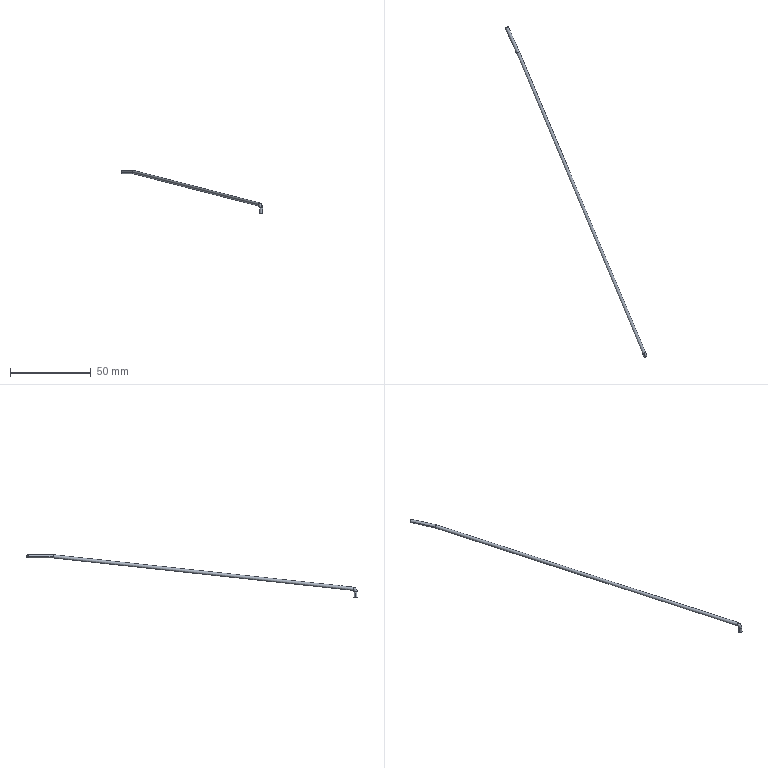Part | STEP file | rear_spoke5 | 1 solid | 10 faces | box 87.859 x 205.125 x 26.5 mm | volume 711.916 mm3 | cylinder 6 | torus 2 | plane 2 | commonest cylinder face diameters 2 x6
STEP:
#1=CARTESIAN_POINT('',(0.,0.,0.));
#2=DIRECTION('',(0.,0.,1.));
#3=DIRECTION('',(1.,0.,0.));
#4=AXIS2_PLACEMENT_3D('',#1,#2,#3);
#5=CARTESIAN_POINT('',(-17.112,24.113,0.3593));
#6=VERTEX_POINT('',#5);
#7=CARTESIAN_POINT('',(-15.725,23.191,0.3593));
#8=VERTEX_POINT('',#7);
#9=CARTESIAN_POINT('',(-16.112,24.113,0.3593));
#10=DIRECTION('',(0.,0.,1.));
#11=DIRECTION('',(1.,0.,0.));
#12=AXIS2_PLACEMENT_3D('',#9,#10,#11);
#13=CIRCLE('',#12,1.);
#14=CARTESIAN_POINT('',(-16.886,25.957,0.3593));
#15=DIRECTION('',(-0.9221,-0.387,0.));
#16=DIRECTION('',(0.387,-0.9221,0.));
#17=AXIS2_PLACEMENT_3D('',#14,#15,#16);
#18=TOROIDAL_SURFACE('',#17,2.,1.);
#19=CARTESIAN_POINT('',(0.,5.11));
#20=DIRECTION('',(0.,-1.));
#21=VECTOR('',#20,1.);
#22=LINE('',#19,#21);
#23=(GEOMETRIC_REPRESENTATION_CONTEXT(2)PARAMETRIC_REPRESENTATION_CONTEXT()REPRESENTATION_CONTEXT('',''));
#24=DEFINITIONAL_REPRESENTATION('',(#22),#23);
#25=PCURVE('',#18,#24);
#26=CARTESIAN_POINT('',(-16.112,24.113,-3.));
#27=DIRECTION('',(0.,0.,1.));
#28=DIRECTION('',(1.,0.,0.));
#29=AXIS2_PLACEMENT_3D('',#26,#27,#28);
#30=CYLINDRICAL_SURFACE('',#29,1.);
#31=CARTESIAN_POINT('',(0.,3.359));
#32=DIRECTION('',(1.,0.));
#33=VECTOR('',#32,1.);
#34=LINE('',#31,#33);
#35=(GEOMETRIC_REPRESENTATION_CONTEXT(2)PARAMETRIC_REPRESENTATION_CONTEXT()REPRESENTATION_CONTEXT('',''));
#36=DEFINITIONAL_REPRESENTATION('',(#34),#35);
#37=PCURVE('',#30,#36);
#38=SURFACE_CURVE('',#13,(#25,#37),.PCURVE_S1.);
#39=EDGE_CURVE('',#6,#8,#38,.T.);
#40=ORIENTED_EDGE('',*,*,#39,.T.);
#41=CARTESIAN_POINT('',(-16.771,25.683,3.345));
#42=VERTEX_POINT('',#41);
#43=CARTESIAN_POINT('',(-16.886,25.957,0.3593));
#44=DIRECTION('',(-0.9221,-0.387,0.));
#45=DIRECTION('',(0.387,-0.9221,0.));
#46=AXIS2_PLACEMENT_3D('',#43,#44,#45);
#47=CIRCLE('',#46,3.);
#48=CARTESIAN_POINT('',(0.,0.));
#49=DIRECTION('',(1.,0.));
#50=VECTOR('',#49,1.);
#51=LINE('',#48,#50);
#52=(GEOMETRIC_REPRESENTATION_CONTEXT(2)PARAMETRIC_REPRESENTATION_CONTEXT()REPRESENTATION_CONTEXT('',''));
#53=DEFINITIONAL_REPRESENTATION('',(#51),#52);
#54=PCURVE('',#18,#53);
#55=CARTESIAN_POINT('',(-16.886,25.957,0.3593));
#56=DIRECTION('',(-0.9221,-0.387,0.));
#57=DIRECTION('',(0.387,-0.9221,0.));
#58=AXIS2_PLACEMENT_3D('',#55,#56,#57);
#59=TOROIDAL_SURFACE('',#58,2.,1.);
#60=CARTESIAN_POINT('',(0.,6.283));
#61=CARTESIAN_POINT('',(0.0223,6.283));
#62=CARTESIAN_POINT('',(0.06689,6.283));
#63=CARTESIAN_POINT('',(0.1338,6.283));
#64=CARTESIAN_POINT('',(0.2007,6.283));
#65=CARTESIAN_POINT('',(0.2675,6.283));
#66=CARTESIAN_POINT('',(0.3344,6.283));
#67=CARTESIAN_POINT('',(0.4013,6.283));
#68=CARTESIAN_POINT('',(0.4682,6.283));
#69=CARTESIAN_POINT('',(0.5351,6.283));
#70=CARTESIAN_POINT('',(0.602,6.283));
#71=CARTESIAN_POINT('',(0.6689,6.283));
#72=CARTESIAN_POINT('',(0.7358,6.283));
#73=CARTESIAN_POINT('',(0.8026,6.283));
#74=CARTESIAN_POINT('',(0.8695,6.283));
#75=CARTESIAN_POINT('',(0.9364,6.283));
#76=CARTESIAN_POINT('',(1.003,6.283));
#77=CARTESIAN_POINT('',(1.07,6.283));
#78=CARTESIAN_POINT('',(1.137,6.283));
#79=CARTESIAN_POINT('',(1.204,6.283));
#80=CARTESIAN_POINT('',(1.271,6.283));
#81=CARTESIAN_POINT('',(1.338,6.283));
#82=CARTESIAN_POINT('',(1.405,6.283));
#83=CARTESIAN_POINT('',(1.449,6.283));
#84=CARTESIAN_POINT('',(1.472,6.283));
#85=B_SPLINE_CURVE_WITH_KNOTS('',3,(#60,#61,#62,#63,#64,#65,#66,#67,#68,#69,#70,#71,#72,#73,#74,#75,#76,#77,#78,#79,#80,#81,#82,#83,#84),.UNSPECIFIED.,.F.,.F.,(4,1,1,1,1,1,1,1,1,1,1,1,1,1,1,1,1,1,1,1,1,1,4),(0.,0.06689,0.1338,0.2007,0.2675,0.3344,0.4013,0.4682,0.5351,0.602,0.6689,0.7358,0.8026,0.8695,0.9364,1.003,1.07,1.137,1.204,1.271,1.338,1.405,1.472),.QUASI_UNIFORM_KNOTS.);
#86=(GEOMETRIC_REPRESENTATION_CONTEXT(2)PARAMETRIC_REPRESENTATION_CONTEXT()REPRESENTATION_CONTEXT('',''));
#87=DEFINITIONAL_REPRESENTATION('',(#85),#86);
#88=PCURVE('',#59,#87);
#89=SURFACE_CURVE('',#47,(#54,#88),.PCURVE_S1.);
#90=EDGE_CURVE('',#8,#42,#89,.T.);
#91=ORIENTED_EDGE('',*,*,#90,.T.);
#92=CARTESIAN_POINT('',(-17.731,25.387,2.349));
#93=VERTEX_POINT('',#92);
#94=CARTESIAN_POINT('',(-16.809,25.774,2.349));
#95=DIRECTION('',(-0.3851,0.9175,0.09911));
#96=DIRECTION('',(0.8651,0.3215,0.3851));
#97=AXIS2_PLACEMENT_3D('',#94,#95,#96);
#98=CIRCLE('',#97,1.);
#99=CARTESIAN_POINT('',(1.472,5.11));
#100=DIRECTION('',(0.,-1.));
#101=VECTOR('',#100,1.);
#102=LINE('',#99,#101);
#103=(GEOMETRIC_REPRESENTATION_CONTEXT(2)PARAMETRIC_REPRESENTATION_CONTEXT()REPRESENTATION_CONTEXT('',''));
#104=DEFINITIONAL_REPRESENTATION('',(#102),#103);
#105=PCURVE('',#18,#104);
#106=CARTESIAN_POINT('',(-16.809,25.774,2.349));
#107=DIRECTION('',(-0.3851,0.9175,0.09911));
#108=DIRECTION('',(-0.9221,-0.387,0.));
#109=AXIS2_PLACEMENT_3D('',#106,#107,#108);
#110=CYLINDRICAL_SURFACE('',#109,1.);
#111=CARTESIAN_POINT('',(-3.539,0.));
#112=DIRECTION('',(1.,0.));
#113=VECTOR('',#112,1.);
#114=LINE('',#111,#113);
#115=(GEOMETRIC_REPRESENTATION_CONTEXT(2)PARAMETRIC_REPRESENTATION_CONTEXT()REPRESENTATION_CONTEXT('',''));
#116=DEFINITIONAL_REPRESENTATION('',(#114),#115);
#117=PCURVE('',#110,#116);
#118=SURFACE_CURVE('',#98,(#105,#117),.PCURVE_S1.);
#119=EDGE_CURVE('',#93,#42,#118,.T.);
#120=ORIENTED_EDGE('',*,*,#119,.F.);
#121=CARTESIAN_POINT('',(-16.847,25.865,1.354));
#122=VERTEX_POINT('',#121);
#123=CARTESIAN_POINT('',(-16.809,25.774,2.349));
#124=DIRECTION('',(-0.3851,0.9175,0.09911));
#125=DIRECTION('',(0.8651,0.3215,0.3851));
#126=AXIS2_PLACEMENT_3D('',#123,#124,#125);
#127=CIRCLE('',#126,1.);
#128=CARTESIAN_POINT('',(1.472,5.11));
#129=DIRECTION('',(0.,-1.));
#130=VECTOR('',#129,1.);
#131=LINE('',#128,#130);
#132=(GEOMETRIC_REPRESENTATION_CONTEXT(2)PARAMETRIC_REPRESENTATION_CONTEXT()REPRESENTATION_CONTEXT('',''));
#133=DEFINITIONAL_REPRESENTATION('',(#131),#132);
#134=PCURVE('',#18,#133);
#135=CARTESIAN_POINT('',(-16.809,25.774,2.349));
#136=DIRECTION('',(-0.3851,0.9175,0.09911));
#137=DIRECTION('',(-0.9221,-0.387,0.));
#138=AXIS2_PLACEMENT_3D('',#135,#136,#137);
#139=CYLINDRICAL_SURFACE('',#138,1.);
#140=CARTESIAN_POINT('',(2.744,0.));
#141=DIRECTION('',(1.,0.));
#142=VECTOR('',#141,1.);
#143=LINE('',#140,#142);
#144=(GEOMETRIC_REPRESENTATION_CONTEXT(2)PARAMETRIC_REPRESENTATION_CONTEXT()REPRESENTATION_CONTEXT('',''));
#145=DEFINITIONAL_REPRESENTATION('',(#143),#144);
#146=PCURVE('',#139,#145);
#147=SURFACE_CURVE('',#127,(#134,#146),.PCURVE_S1.);
#148=EDGE_CURVE('',#122,#93,#147,.T.);
#149=ORIENTED_EDGE('',*,*,#148,.F.);
#150=CARTESIAN_POINT('',(-16.499,25.035,0.3593));
#151=VERTEX_POINT('',#150);
#152=CARTESIAN_POINT('',(-16.886,25.957,0.3593));
#153=DIRECTION('',(-0.9221,-0.387,0.));
#154=DIRECTION('',(0.387,-0.9221,0.));
#155=AXIS2_PLACEMENT_3D('',#152,#153,#154);
#156=CIRCLE('',#155,1.);
#157=CARTESIAN_POINT('',(0.,3.142));
#158=DIRECTION('',(1.,0.));
#159=VECTOR('',#158,1.);
#160=LINE('',#157,#159);
#161=(GEOMETRIC_REPRESENTATION_CONTEXT(2)PARAMETRIC_REPRESENTATION_CONTEXT()REPRESENTATION_CONTEXT('',''));
#162=DEFINITIONAL_REPRESENTATION('',(#160),#161);
#163=PCURVE('',#18,#162);
#164=CARTESIAN_POINT('',(0.,3.142));
#165=DIRECTION('',(1.,0.));
#166=VECTOR('',#165,1.);
#167=LINE('',#164,#166);
#168=(GEOMETRIC_REPRESENTATION_CONTEXT(2)PARAMETRIC_REPRESENTATION_CONTEXT()REPRESENTATION_CONTEXT('',''));
#169=DEFINITIONAL_REPRESENTATION('',(#167),#168);
#170=PCURVE('',#59,#169);
#171=SURFACE_CURVE('',#156,(#163,#170),.PCURVE_S1.);
#172=EDGE_CURVE('',#151,#122,#171,.T.);
#173=ORIENTED_EDGE('',*,*,#172,.F.);
#174=CARTESIAN_POINT('',(-16.112,24.113,0.3593));
#175=DIRECTION('',(0.,0.,1.));
#176=DIRECTION('',(1.,0.,0.));
#177=AXIS2_PLACEMENT_3D('',#174,#175,#176);
#178=CIRCLE('',#177,1.);
#179=CARTESIAN_POINT('',(0.,5.11));
#180=DIRECTION('',(0.,-1.));
#181=VECTOR('',#180,1.);
#182=LINE('',#179,#181);
#183=(GEOMETRIC_REPRESENTATION_CONTEXT(2)PARAMETRIC_REPRESENTATION_CONTEXT()REPRESENTATION_CONTEXT('',''));
#184=DEFINITIONAL_REPRESENTATION('',(#182),#183);
#185=PCURVE('',#18,#184);
#186=CARTESIAN_POINT('',(-16.112,24.113,-3.));
#187=DIRECTION('',(0.,0.,1.));
#188=DIRECTION('',(1.,0.,0.));
#189=AXIS2_PLACEMENT_3D('',#186,#187,#188);
#190=CYLINDRICAL_SURFACE('',#189,1.);
#191=CARTESIAN_POINT('',(0.,3.359));
#192=DIRECTION('',(1.,0.));
#193=VECTOR('',#192,1.);
#194=LINE('',#191,#193);
#195=(GEOMETRIC_REPRESENTATION_CONTEXT(2)PARAMETRIC_REPRESENTATION_CONTEXT()REPRESENTATION_CONTEXT('',''));
#196=DEFINITIONAL_REPRESENTATION('',(#194),#195);
#197=PCURVE('',#190,#196);
#198=SURFACE_CURVE('',#178,(#185,#197),.PCURVE_S1.);
#199=EDGE_CURVE('',#151,#6,#198,.T.);
#200=ORIENTED_EDGE('',*,*,#199,.T.);
#201=EDGE_LOOP('',(#40,#91,#120,#149,#173,#200));
#202=FACE_BOUND('',#201,.T.);
#203=ADVANCED_FACE('',(#202),#18,.T.);
#204=ORIENTED_EDGE('',*,*,#119,.T.);
#205=CARTESIAN_POINT('',(-15.887,26.161,2.349));
#206=VERTEX_POINT('',#205);
#207=CARTESIAN_POINT('',(-16.809,25.774,2.349));
#208=DIRECTION('',(-0.3851,0.9175,0.09911));
#209=DIRECTION('',(0.8651,0.3215,0.3851));
#210=AXIS2_PLACEMENT_3D('',#207,#208,#209);
#211=CIRCLE('',#210,1.);
#212=CARTESIAN_POINT('',(-3.539,0.));
#213=DIRECTION('',(1.,0.));
#214=VECTOR('',#213,1.);
#215=LINE('',#212,#214);
#216=(GEOMETRIC_REPRESENTATION_CONTEXT(2)PARAMETRIC_REPRESENTATION_CONTEXT()REPRESENTATION_CONTEXT('',''));
#217=DEFINITIONAL_REPRESENTATION('',(#215),#216);
#218=PCURVE('',#110,#217);
#219=CARTESIAN_POINT('',(1.472,11.393));
#220=DIRECTION('',(0.,-1.));
#221=VECTOR('',#220,1.);
#222=LINE('',#219,#221);
#223=(GEOMETRIC_REPRESENTATION_CONTEXT(2)PARAMETRIC_REPRESENTATION_CONTEXT()REPRESENTATION_CONTEXT('',''));
#224=DEFINITIONAL_REPRESENTATION('',(#222),#223);
#225=PCURVE('',#59,#224);
#226=SURFACE_CURVE('',#211,(#218,#225),.PCURVE_S1.);
#227=EDGE_CURVE('',#42,#206,#226,.T.);
#228=ORIENTED_EDGE('',*,*,#227,.T.);
#229=CARTESIAN_POINT('',(-94.191,212.713,22.501));
#230=VERTEX_POINT('',#229);
#231=CARTESIAN_POINT('',(-15.887,26.161,2.349));
#232=DIRECTION('',(-0.3851,0.9175,0.09911));
#233=VECTOR('',#232,1.);
#234=LINE('',#231,#233);
#235=CARTESIAN_POINT('',(3.142,0.));
#236=DIRECTION('',(0.,1.));
#237=VECTOR('',#236,1.);
#238=LINE('',#235,#237);
#239=(GEOMETRIC_REPRESENTATION_CONTEXT(2)PARAMETRIC_REPRESENTATION_CONTEXT()REPRESENTATION_CONTEXT('',''));
#240=DEFINITIONAL_REPRESENTATION('',(#238),#239);
#241=PCURVE('',#110,#240);
#242=CARTESIAN_POINT('',(3.142,0.));
#243=DIRECTION('',(0.,1.));
#244=VECTOR('',#243,1.);
#245=LINE('',#242,#244);
#246=(GEOMETRIC_REPRESENTATION_CONTEXT(2)PARAMETRIC_REPRESENTATION_CONTEXT()REPRESENTATION_CONTEXT('',''));
#247=DEFINITIONAL_REPRESENTATION('',(#245),#246);
#248=PCURVE('',#139,#247);
#249=SURFACE_CURVE('',#234,(#241,#248),.PCURVE_S1.);
#250=EDGE_CURVE('',#206,#230,#249,.T.);
#251=ORIENTED_EDGE('',*,*,#250,.T.);
#252=CARTESIAN_POINT('',(-96.026,211.917,22.5));
#253=VERTEX_POINT('',#252);
#254=CARTESIAN_POINT('',(-94.191,212.713,22.501));
#255=CARTESIAN_POINT('',(-94.152,212.622,24.499));
#256=CARTESIAN_POINT('',(-95.985,211.827,24.498));
#257=CARTESIAN_POINT('',(-96.026,211.917,22.5));
#258=(BOUNDED_CURVE()B_SPLINE_CURVE(3,(#254,#255,#256,#257),.UNSPECIFIED.,.F.,.F.)B_SPLINE_CURVE_WITH_KNOTS((4,4),(4.948,8.088),.PIECEWISE_BEZIER_KNOTS.)CURVE()GEOMETRIC_REPRESENTATION_ITEM()RATIONAL_B_SPLINE_CURVE((1.,0.3337,0.3337,1.))REPRESENTATION_ITEM(''));
#259=CARTESIAN_POINT('',(3.142,203.321));
#260=CARTESIAN_POINT('',(3.111,203.322));
#261=CARTESIAN_POINT('',(3.048,203.325));
#262=CARTESIAN_POINT('',(2.944,203.33));
#263=CARTESIAN_POINT('',(2.83,203.335));
#264=CARTESIAN_POINT('',(2.706,203.341));
#265=CARTESIAN_POINT('',(2.571,203.346));
#266=CARTESIAN_POINT('',(2.426,203.351));
#267=CARTESIAN_POINT('',(2.27,203.355));
#268=CARTESIAN_POINT('',(2.105,203.358));
#269=CARTESIAN_POINT('',(1.932,203.36));
#270=CARTESIAN_POINT('',(1.753,203.36));
#271=CARTESIAN_POINT('',(1.571,203.359));
#272=CARTESIAN_POINT('',(1.39,203.356));
#273=CARTESIAN_POINT('',(1.211,203.351));
#274=CARTESIAN_POINT('',(1.038,203.346));
#275=CARTESIAN_POINT('',(0.8727,203.339));
#276=CARTESIAN_POINT('',(0.7168,203.333));
#277=CARTESIAN_POINT('',(0.5714,203.326));
#278=CARTESIAN_POINT('',(0.4367,203.319));
#279=CARTESIAN_POINT('',(0.3126,203.313));
#280=CARTESIAN_POINT('',(0.1989,203.307));
#281=CARTESIAN_POINT('',(0.09484,203.302));
#282=CARTESIAN_POINT('',(0.03148,203.298));
#283=CARTESIAN_POINT('',(0.00118,203.297));
#284=B_SPLINE_CURVE_WITH_KNOTS('',3,(#259,#260,#261,#262,#263,#264,#265,#266,#267,#268,#269,#270,#271,#272,#273,#274,#275,#276,#277,#278,#279,#280,#281,#282,#283),.UNSPECIFIED.,.F.,.F.,(4,1,1,1,1,1,1,1,1,1,1,1,1,1,1,1,1,1,1,1,1,1,4),(4.948,5.09,5.233,5.376,5.519,5.661,5.804,5.947,6.09,6.232,6.375,6.518,6.661,6.803,6.946,7.089,7.232,7.374,7.517,7.66,7.802,7.945,8.088),.QUASI_UNIFORM_KNOTS.);
#285=(GEOMETRIC_REPRESENTATION_CONTEXT(2)PARAMETRIC_REPRESENTATION_CONTEXT()REPRESENTATION_CONTEXT('',''));
#286=DEFINITIONAL_REPRESENTATION('',(#284),#285);
#287=PCURVE('',#110,#286);
#288=CARTESIAN_POINT('',(-95.017,212.111,22.5));
#289=DIRECTION('',(-0.4088,0.9126,0.));
#290=DIRECTION('',(-0.9126,-0.4088,0.));
#291=AXIS2_PLACEMENT_3D('',#288,#289,#290);
#292=CYLINDRICAL_SURFACE('',#291,1.);
#293=CARTESIAN_POINT('',(3.14,0.2119));
#294=CARTESIAN_POINT('',(3.11,0.2104));
#295=CARTESIAN_POINT('',(3.047,0.2073));
#296=CARTESIAN_POINT('',(2.943,0.2024));
#297=CARTESIAN_POINT('',(2.829,0.1972));
#298=CARTESIAN_POINT('',(2.705,0.192));
#299=CARTESIAN_POINT('',(2.57,0.1869));
#300=CARTESIAN_POINT('',(2.425,0.1821));
#301=CARTESIAN_POINT('',(2.269,0.178));
#302=CARTESIAN_POINT('',(2.104,0.1748));
#303=CARTESIAN_POINT('',(1.931,0.1729));
#304=CARTESIAN_POINT('',(1.752,0.1726));
#305=CARTESIAN_POINT('',(1.57,0.1739));
#306=CARTESIAN_POINT('',(1.388,0.1769));
#307=CARTESIAN_POINT('',(1.21,0.1813));
#308=CARTESIAN_POINT('',(1.037,0.1869));
#309=CARTESIAN_POINT('',(0.8715,0.1933));
#310=CARTESIAN_POINT('',(0.7157,0.2001));
#311=CARTESIAN_POINT('',(0.5702,0.2069));
#312=CARTESIAN_POINT('',(0.4355,0.2136));
#313=CARTESIAN_POINT('',(0.3115,0.2199));
#314=CARTESIAN_POINT('',(0.1977,0.2257));
#315=CARTESIAN_POINT('',(0.09366,0.231));
#316=CARTESIAN_POINT('',(0.0303,0.2342));
#317=CARTESIAN_POINT('',(0.,0.2357));
#318=B_SPLINE_CURVE_WITH_KNOTS('',3,(#293,#294,#295,#296,#297,#298,#299,#300,#301,#302,#303,#304,#305,#306,#307,#308,#309,#310,#311,#312,#313,#314,#315,#316,#317),.UNSPECIFIED.,.F.,.F.,(4,1,1,1,1,1,1,1,1,1,1,1,1,1,1,1,1,1,1,1,1,1,4),(4.948,5.09,5.233,5.376,5.519,5.661,5.804,5.947,6.09,6.232,6.375,6.518,6.661,6.803,6.946,7.089,7.232,7.374,7.517,7.66,7.802,7.945,8.088),.QUASI_UNIFORM_KNOTS.);
#319=(GEOMETRIC_REPRESENTATION_CONTEXT(2)PARAMETRIC_REPRESENTATION_CONTEXT()REPRESENTATION_CONTEXT('',''));
#320=DEFINITIONAL_REPRESENTATION('',(#318),#319);
#321=PCURVE('',#292,#320);
#322=SURFACE_CURVE('',#258,(#287,#321),.PCURVE_S1.);
#323=EDGE_CURVE('',#230,#253,#322,.T.);
#324=ORIENTED_EDGE('',*,*,#323,.T.);
#325=CARTESIAN_POINT('',(-96.026,211.917,22.499));
#326=VERTEX_POINT('',#325);
#327=CARTESIAN_POINT('',(-96.026,211.917,22.5));
#328=CARTESIAN_POINT('',(-96.026,211.917,22.5));
#329=CARTESIAN_POINT('',(-96.026,211.917,22.499));
#330=CARTESIAN_POINT('',(-96.026,211.917,22.499));
#331=(BOUNDED_CURVE()B_SPLINE_CURVE(3,(#327,#328,#329,#330),.UNSPECIFIED.,.F.,.F.)B_SPLINE_CURVE_WITH_KNOTS((4,4),(1.805,1.806),.PIECEWISE_BEZIER_KNOTS.)CURVE()GEOMETRIC_REPRESENTATION_ITEM()RATIONAL_B_SPLINE_CURVE((1.,1.,1.,1.))REPRESENTATION_ITEM(''));
#332=CARTESIAN_POINT('',(0.00118,203.297));
#333=CARTESIAN_POINT('',(0.,203.297));
#334=B_SPLINE_CURVE_WITH_KNOTS('',1,(#332,#333),.UNSPECIFIED.,.F.,.F.,(2,2),(1.805,1.806),.PIECEWISE_BEZIER_KNOTS.);
#335=(GEOMETRIC_REPRESENTATION_CONTEXT(2)PARAMETRIC_REPRESENTATION_CONTEXT()REPRESENTATION_CONTEXT('',''));
#336=DEFINITIONAL_REPRESENTATION('',(#334),#335);
#337=PCURVE('',#110,#336);
#338=CARTESIAN_POINT('',(-95.017,212.111,22.5));
#339=DIRECTION('',(-0.4088,0.9126,0.));
#340=DIRECTION('',(-0.9126,-0.4088,0.));
#341=AXIS2_PLACEMENT_3D('',#338,#339,#340);
#342=CYLINDRICAL_SURFACE('',#341,1.);
#343=CARTESIAN_POINT('',(6.283,0.2357));
#344=CARTESIAN_POINT('',(6.282,0.2357));
#345=B_SPLINE_CURVE_WITH_KNOTS('',1,(#343,#344),.UNSPECIFIED.,.F.,.F.,(2,2),(1.805,1.806),.PIECEWISE_BEZIER_KNOTS.);
#346=(GEOMETRIC_REPRESENTATION_CONTEXT(2)PARAMETRIC_REPRESENTATION_CONTEXT()REPRESENTATION_CONTEXT('',''));
#347=DEFINITIONAL_REPRESENTATION('',(#345),#346);
#348=PCURVE('',#342,#347);
#349=SURFACE_CURVE('',#331,(#337,#348),.PCURVE_S1.);
#350=EDGE_CURVE('',#253,#326,#349,.T.);
#351=ORIENTED_EDGE('',*,*,#350,.T.);
#352=CARTESIAN_POINT('',(-17.731,25.387,2.349));
#353=DIRECTION('',(-0.3851,0.9175,0.09911));
#354=VECTOR('',#353,1.);
#355=LINE('',#352,#354);
#356=CARTESIAN_POINT('',(0.,0.));
#357=DIRECTION('',(0.,1.));
#358=VECTOR('',#357,1.);
#359=LINE('',#356,#358);
#360=(GEOMETRIC_REPRESENTATION_CONTEXT(2)PARAMETRIC_REPRESENTATION_CONTEXT()REPRESENTATION_CONTEXT('',''));
#361=DEFINITIONAL_REPRESENTATION('',(#359),#360);
#362=PCURVE('',#110,#361);
#363=CARTESIAN_POINT('',(6.283,0.));
#364=DIRECTION('',(0.,1.));
#365=VECTOR('',#364,1.);
#366=LINE('',#363,#365);
#367=(GEOMETRIC_REPRESENTATION_CONTEXT(2)PARAMETRIC_REPRESENTATION_CONTEXT()REPRESENTATION_CONTEXT('',''));
#368=DEFINITIONAL_REPRESENTATION('',(#366),#367);
#369=PCURVE('',#139,#368);
#370=SURFACE_CURVE('',#355,(#362,#369),.PCURVE_S1.);
#371=EDGE_CURVE('',#93,#326,#370,.T.);
#372=ORIENTED_EDGE('',*,*,#371,.F.);
#373=EDGE_LOOP('',(#204,#228,#251,#324,#351,#372));
#374=FACE_BOUND('',#373,.T.);
#375=ADVANCED_FACE('',(#374),#110,.T.);
#376=CARTESIAN_POINT('',(-15.112,24.113,-3.));
#377=VERTEX_POINT('',#376);
#378=CARTESIAN_POINT('',(-17.112,24.113,-3.));
#379=VERTEX_POINT('',#378);
#380=CARTESIAN_POINT('',(-16.112,24.113,-3.));
#381=DIRECTION('',(0.,0.,1.));
#382=DIRECTION('',(1.,0.,0.));
#383=AXIS2_PLACEMENT_3D('',#380,#381,#382);
#384=CIRCLE('',#383,1.);
#385=CARTESIAN_POINT('',(0.,0.));
#386=DIRECTION('',(1.,0.));
#387=VECTOR('',#386,1.);
#388=LINE('',#385,#387);
#389=(GEOMETRIC_REPRESENTATION_CONTEXT(2)PARAMETRIC_REPRESENTATION_CONTEXT()REPRESENTATION_CONTEXT('',''));
#390=DEFINITIONAL_REPRESENTATION('',(#388),#389);
#391=PCURVE('',#190,#390);
#392=CARTESIAN_POINT('',(-16.112,24.113,-3.));
#393=DIRECTION('',(0.,0.,1.));
#394=DIRECTION('',(1.,0.,0.));
#395=AXIS2_PLACEMENT_3D('',#392,#393,#394);
#396=PLANE('',#395);
#397=CARTESIAN_POINT('',(0.,0.));
#398=DIRECTION('',(1.,0.));
#399=AXIS2_PLACEMENT_2D('',#397,#398);
#400=CIRCLE('',#399,1.);
#401=(GEOMETRIC_REPRESENTATION_CONTEXT(2)PARAMETRIC_REPRESENTATION_CONTEXT()REPRESENTATION_CONTEXT('',''));
#402=DEFINITIONAL_REPRESENTATION('',(#400),#401);
#403=PCURVE('',#396,#402);
#404=SURFACE_CURVE('',#384,(#391,#403),.PCURVE_S1.);
#405=EDGE_CURVE('',#377,#379,#404,.T.);
#406=ORIENTED_EDGE('',*,*,#405,.T.);
#407=CARTESIAN_POINT('',(-17.112,24.113,-3.));
#408=DIRECTION('',(0.,0.,1.));
#409=VECTOR('',#408,1.);
#410=LINE('',#407,#409);
#411=CARTESIAN_POINT('',(3.142,0.));
#412=DIRECTION('',(0.,1.));
#413=VECTOR('',#412,1.);
#414=LINE('',#411,#413);
#415=(GEOMETRIC_REPRESENTATION_CONTEXT(2)PARAMETRIC_REPRESENTATION_CONTEXT()REPRESENTATION_CONTEXT('',''));
#416=DEFINITIONAL_REPRESENTATION('',(#414),#415);
#417=PCURVE('',#190,#416);
#418=CARTESIAN_POINT('',(3.142,0.));
#419=DIRECTION('',(0.,1.));
#420=VECTOR('',#419,1.);
#421=LINE('',#418,#420);
#422=(GEOMETRIC_REPRESENTATION_CONTEXT(2)PARAMETRIC_REPRESENTATION_CONTEXT()REPRESENTATION_CONTEXT('',''));
#423=DEFINITIONAL_REPRESENTATION('',(#421),#422);
#424=PCURVE('',#30,#423);
#425=SURFACE_CURVE('',#410,(#417,#424),.PCURVE_S1.);
#426=EDGE_CURVE('',#379,#6,#425,.T.);
#427=ORIENTED_EDGE('',*,*,#426,.T.);
#428=ORIENTED_EDGE('',*,*,#199,.F.);
#429=CARTESIAN_POINT('',(-15.112,24.113,0.3593));
#430=VERTEX_POINT('',#429);
#431=CARTESIAN_POINT('',(-16.112,24.113,0.3593));
#432=DIRECTION('',(0.,0.,1.));
#433=DIRECTION('',(1.,0.,0.));
#434=AXIS2_PLACEMENT_3D('',#431,#432,#433);
#435=CIRCLE('',#434,1.);
#436=CARTESIAN_POINT('',(0.,3.359));
#437=DIRECTION('',(1.,0.));
#438=VECTOR('',#437,1.);
#439=LINE('',#436,#438);
#440=(GEOMETRIC_REPRESENTATION_CONTEXT(2)PARAMETRIC_REPRESENTATION_CONTEXT()REPRESENTATION_CONTEXT('',''));
#441=DEFINITIONAL_REPRESENTATION('',(#439),#440);
#442=PCURVE('',#190,#441);
#443=CARTESIAN_POINT('',(0.,5.11));
#444=DIRECTION('',(0.,-1.));
#445=VECTOR('',#444,1.);
#446=LINE('',#443,#445);
#447=(GEOMETRIC_REPRESENTATION_CONTEXT(2)PARAMETRIC_REPRESENTATION_CONTEXT()REPRESENTATION_CONTEXT('',''));
#448=DEFINITIONAL_REPRESENTATION('',(#446),#447);
#449=PCURVE('',#59,#448);
#450=SURFACE_CURVE('',#435,(#442,#449),.PCURVE_S1.);
#451=EDGE_CURVE('',#430,#151,#450,.T.);
#452=ORIENTED_EDGE('',*,*,#451,.F.);
#453=CARTESIAN_POINT('',(-15.112,24.113,-3.));
#454=DIRECTION('',(0.,0.,1.));
#455=VECTOR('',#454,1.);
#456=LINE('',#453,#455);
#457=CARTESIAN_POINT('',(0.,0.));
#458=DIRECTION('',(0.,1.));
#459=VECTOR('',#458,1.);
#460=LINE('',#457,#459);
#461=(GEOMETRIC_REPRESENTATION_CONTEXT(2)PARAMETRIC_REPRESENTATION_CONTEXT()REPRESENTATION_CONTEXT('',''));
#462=DEFINITIONAL_REPRESENTATION('',(#460),#461);
#463=PCURVE('',#190,#462);
#464=CARTESIAN_POINT('',(6.283,0.));
#465=DIRECTION('',(0.,1.));
#466=VECTOR('',#465,1.);
#467=LINE('',#464,#466);
#468=(GEOMETRIC_REPRESENTATION_CONTEXT(2)PARAMETRIC_REPRESENTATION_CONTEXT()REPRESENTATION_CONTEXT('',''));
#469=DEFINITIONAL_REPRESENTATION('',(#467),#468);
#470=PCURVE('',#30,#469);
#471=SURFACE_CURVE('',#456,(#463,#470),.PCURVE_S1.);
#472=EDGE_CURVE('',#377,#430,#471,.T.);
#473=ORIENTED_EDGE('',*,*,#472,.F.);
#474=EDGE_LOOP('',(#406,#427,#428,#452,#473));
#475=FACE_BOUND('',#474,.T.);
#476=ADVANCED_FACE('',(#475),#190,.T.);
#477=CARTESIAN_POINT('',(-94.191,212.713,22.5));
#478=VERTEX_POINT('',#477);
#479=CARTESIAN_POINT('',(-94.191,212.713,22.5));
#480=CARTESIAN_POINT('',(-94.191,212.713,22.5));
#481=CARTESIAN_POINT('',(-94.191,212.713,22.501));
#482=CARTESIAN_POINT('',(-94.191,212.713,22.501));
#483=(BOUNDED_CURVE()B_SPLINE_CURVE(3,(#479,#480,#481,#482),.UNSPECIFIED.,.F.,.F.)B_SPLINE_CURVE_WITH_KNOTS((4,4),(4.946,4.948),.PIECEWISE_BEZIER_KNOTS.)CURVE()GEOMETRIC_REPRESENTATION_ITEM()RATIONAL_B_SPLINE_CURVE((1.,1.,1.,1.))REPRESENTATION_ITEM(''));
#484=CARTESIAN_POINT('',(3.142,0.212));
#485=CARTESIAN_POINT('',(3.14,0.2119));
#486=B_SPLINE_CURVE_WITH_KNOTS('',1,(#484,#485),.UNSPECIFIED.,.F.,.F.,(2,2),(4.946,4.948),.PIECEWISE_BEZIER_KNOTS.);
#487=(GEOMETRIC_REPRESENTATION_CONTEXT(2)PARAMETRIC_REPRESENTATION_CONTEXT()REPRESENTATION_CONTEXT('',''));
#488=DEFINITIONAL_REPRESENTATION('',(#486),#487);
#489=PCURVE('',#292,#488);
#490=CARTESIAN_POINT('',(3.143,203.321));
#491=CARTESIAN_POINT('',(3.142,203.321));
#492=B_SPLINE_CURVE_WITH_KNOTS('',1,(#490,#491),.UNSPECIFIED.,.F.,.F.,(2,2),(4.946,4.948),.PIECEWISE_BEZIER_KNOTS.);
#493=(GEOMETRIC_REPRESENTATION_CONTEXT(2)PARAMETRIC_REPRESENTATION_CONTEXT()REPRESENTATION_CONTEXT('',''));
#494=DEFINITIONAL_REPRESENTATION('',(#492),#493);
#495=PCURVE('',#139,#494);
#496=SURFACE_CURVE('',#483,(#489,#495),.PCURVE_S1.);
#497=EDGE_CURVE('',#478,#230,#496,.T.);
#498=ORIENTED_EDGE('',*,*,#497,.F.);
#499=CARTESIAN_POINT('',(-101.145,228.237,22.5));
#500=VERTEX_POINT('',#499);
#501=CARTESIAN_POINT('',(-94.104,212.52,22.5));
#502=DIRECTION('',(-0.4088,0.9126,0.));
#503=VECTOR('',#502,1.);
#504=LINE('',#501,#503);
#505=CARTESIAN_POINT('',(3.142,0.));
#506=DIRECTION('',(0.,1.));
#507=VECTOR('',#506,1.);
#508=LINE('',#505,#507);
#509=(GEOMETRIC_REPRESENTATION_CONTEXT(2)PARAMETRIC_REPRESENTATION_CONTEXT()REPRESENTATION_CONTEXT('',''));
#510=DEFINITIONAL_REPRESENTATION('',(#508),#509);
#511=PCURVE('',#292,#510);
#512=CARTESIAN_POINT('',(3.142,0.));
#513=DIRECTION('',(0.,1.));
#514=VECTOR('',#513,1.);
#515=LINE('',#512,#514);
#516=(GEOMETRIC_REPRESENTATION_CONTEXT(2)PARAMETRIC_REPRESENTATION_CONTEXT()REPRESENTATION_CONTEXT('',''));
#517=DEFINITIONAL_REPRESENTATION('',(#515),#516);
#518=PCURVE('',#342,#517);
#519=SURFACE_CURVE('',#504,(#511,#518),.PCURVE_S1.);
#520=EDGE_CURVE('',#478,#500,#519,.T.);
#521=ORIENTED_EDGE('',*,*,#520,.T.);
#522=CARTESIAN_POINT('',(-102.97,227.42,22.5));
#523=VERTEX_POINT('',#522);
#524=CARTESIAN_POINT('',(-102.057,227.828,22.5));
#525=DIRECTION('',(-0.4088,0.9126,0.));
#526=DIRECTION('',(0.8411,0.3768,0.3881));
#527=AXIS2_PLACEMENT_3D('',#524,#525,#526);
#528=CIRCLE('',#527,1.);
#529=CARTESIAN_POINT('',(-3.54,17.222));
#530=DIRECTION('',(1.,0.));
#531=VECTOR('',#530,1.);
#532=LINE('',#529,#531);
#533=(GEOMETRIC_REPRESENTATION_CONTEXT(2)PARAMETRIC_REPRESENTATION_CONTEXT()REPRESENTATION_CONTEXT('',''));
#534=DEFINITIONAL_REPRESENTATION('',(#532),#533);
#535=PCURVE('',#292,#534);
#536=CARTESIAN_POINT('',(-102.057,227.828,22.5));
#537=DIRECTION('',(-0.4088,0.9126,0.));
#538=DIRECTION('',(0.8411,0.3768,0.3881));
#539=AXIS2_PLACEMENT_3D('',#536,#537,#538);
#540=PLANE('',#539);
#541=CARTESIAN_POINT('',(0.,0.));
#542=DIRECTION('',(1.,0.));
#543=AXIS2_PLACEMENT_2D('',#541,#542);
#544=CIRCLE('',#543,1.);
#545=(GEOMETRIC_REPRESENTATION_CONTEXT(2)PARAMETRIC_REPRESENTATION_CONTEXT()REPRESENTATION_CONTEXT('',''));
#546=DEFINITIONAL_REPRESENTATION('',(#544),#545);
#547=PCURVE('',#540,#546);
#548=SURFACE_CURVE('',#528,(#535,#547),.PCURVE_S1.);
#549=EDGE_CURVE('',#523,#500,#548,.T.);
#550=ORIENTED_EDGE('',*,*,#549,.F.);
#551=CARTESIAN_POINT('',(-95.929,211.702,22.5));
#552=DIRECTION('',(-0.4088,0.9126,0.));
#553=VECTOR('',#552,1.);
#554=LINE('',#551,#553);
#555=CARTESIAN_POINT('',(0.,0.));
#556=DIRECTION('',(0.,1.));
#557=VECTOR('',#556,1.);
#558=LINE('',#555,#557);
#559=(GEOMETRIC_REPRESENTATION_CONTEXT(2)PARAMETRIC_REPRESENTATION_CONTEXT()REPRESENTATION_CONTEXT('',''));
#560=DEFINITIONAL_REPRESENTATION('',(#558),#559);
#561=PCURVE('',#292,#560);
#562=CARTESIAN_POINT('',(6.283,0.));
#563=DIRECTION('',(0.,1.));
#564=VECTOR('',#563,1.);
#565=LINE('',#562,#564);
#566=(GEOMETRIC_REPRESENTATION_CONTEXT(2)PARAMETRIC_REPRESENTATION_CONTEXT()REPRESENTATION_CONTEXT('',''));
#567=DEFINITIONAL_REPRESENTATION('',(#565),#566);
#568=PCURVE('',#342,#567);
#569=SURFACE_CURVE('',#554,(#561,#568),.PCURVE_S1.);
#570=EDGE_CURVE('',#253,#523,#569,.T.);
#571=ORIENTED_EDGE('',*,*,#570,.F.);
#572=ORIENTED_EDGE('',*,*,#323,.F.);
#573=EDGE_LOOP('',(#498,#521,#550,#571,#572));
#574=FACE_BOUND('',#573,.T.);
#575=ADVANCED_FACE('',(#574),#292,.T.);
#576=ORIENTED_EDGE('',*,*,#250,.F.);
#577=CARTESIAN_POINT('',(-16.809,25.774,2.349));
#578=DIRECTION('',(-0.3851,0.9175,0.09911));
#579=DIRECTION('',(0.8651,0.3215,0.3851));
#580=AXIS2_PLACEMENT_3D('',#577,#578,#579);
#581=CIRCLE('',#580,1.);
#582=CARTESIAN_POINT('',(2.744,0.));
#583=DIRECTION('',(1.,0.));
#584=VECTOR('',#583,1.);
#585=LINE('',#582,#584);
#586=(GEOMETRIC_REPRESENTATION_CONTEXT(2)PARAMETRIC_REPRESENTATION_CONTEXT()REPRESENTATION_CONTEXT('',''));
#587=DEFINITIONAL_REPRESENTATION('',(#585),#586);
#588=PCURVE('',#139,#587);
#589=CARTESIAN_POINT('',(1.472,5.11));
#590=DIRECTION('',(0.,-1.));
#591=VECTOR('',#590,1.);
#592=LINE('',#589,#591);
#593=(GEOMETRIC_REPRESENTATION_CONTEXT(2)PARAMETRIC_REPRESENTATION_CONTEXT()REPRESENTATION_CONTEXT('',''));
#594=DEFINITIONAL_REPRESENTATION('',(#592),#593);
#595=PCURVE('',#59,#594);
#596=SURFACE_CURVE('',#581,(#588,#595),.PCURVE_S1.);
#597=EDGE_CURVE('',#206,#122,#596,.T.);
#598=ORIENTED_EDGE('',*,*,#597,.T.);
#599=ORIENTED_EDGE('',*,*,#148,.T.);
#600=ORIENTED_EDGE('',*,*,#371,.T.);
#601=CARTESIAN_POINT('',(-96.026,211.917,22.499));
#602=CARTESIAN_POINT('',(-96.064,212.009,20.501));
#603=CARTESIAN_POINT('',(-94.231,212.804,20.502));
#604=CARTESIAN_POINT('',(-94.191,212.713,22.5));
#605=(BOUNDED_CURVE()B_SPLINE_CURVE(3,(#601,#602,#603,#604),.UNSPECIFIED.,.F.,.F.)B_SPLINE_CURVE_WITH_KNOTS((4,4),(1.806,4.946),.PIECEWISE_BEZIER_KNOTS.)CURVE()GEOMETRIC_REPRESENTATION_ITEM()RATIONAL_B_SPLINE_CURVE((1.,0.3337,0.3337,1.))REPRESENTATION_ITEM(''));
#606=CARTESIAN_POINT('',(6.283,203.297));
#607=CARTESIAN_POINT('',(6.253,203.295));
#608=CARTESIAN_POINT('',(6.19,203.292));
#609=CARTESIAN_POINT('',(6.085,203.287));
#610=CARTESIAN_POINT('',(5.972,203.282));
#611=CARTESIAN_POINT('',(5.848,203.277));
#612=CARTESIAN_POINT('',(5.713,203.272));
#613=CARTESIAN_POINT('',(5.568,203.267));
#614=CARTESIAN_POINT('',(5.412,203.263));
#615=CARTESIAN_POINT('',(5.246,203.26));
#616=CARTESIAN_POINT('',(5.073,203.258));
#617=CARTESIAN_POINT('',(4.895,203.258));
#618=CARTESIAN_POINT('',(4.713,203.259));
#619=CARTESIAN_POINT('',(4.531,203.262));
#620=CARTESIAN_POINT('',(4.353,203.266));
#621=CARTESIAN_POINT('',(4.179,203.272));
#622=CARTESIAN_POINT('',(4.014,203.278));
#623=CARTESIAN_POINT('',(3.858,203.285));
#624=CARTESIAN_POINT('',(3.713,203.292));
#625=CARTESIAN_POINT('',(3.578,203.299));
#626=CARTESIAN_POINT('',(3.454,203.305));
#627=CARTESIAN_POINT('',(3.34,203.311));
#628=CARTESIAN_POINT('',(3.236,203.316));
#629=CARTESIAN_POINT('',(3.173,203.319));
#630=CARTESIAN_POINT('',(3.143,203.321));
#631=B_SPLINE_CURVE_WITH_KNOTS('',3,(#606,#607,#608,#609,#610,#611,#612,#613,#614,#615,#616,#617,#618,#619,#620,#621,#622,#623,#624,#625,#626,#627,#628,#629,#630),.UNSPECIFIED.,.F.,.F.,(4,1,1,1,1,1,1,1,1,1,1,1,1,1,1,1,1,1,1,1,1,1,4),(1.806,1.949,2.091,2.234,2.377,2.52,2.662,2.805,2.948,3.091,3.233,3.376,3.519,3.662,3.804,3.947,4.09,4.233,4.375,4.518,4.661,4.804,4.946),.QUASI_UNIFORM_KNOTS.);
#632=(GEOMETRIC_REPRESENTATION_CONTEXT(2)PARAMETRIC_REPRESENTATION_CONTEXT()REPRESENTATION_CONTEXT('',''));
#633=DEFINITIONAL_REPRESENTATION('',(#631),#632);
#634=PCURVE('',#139,#633);
#635=CARTESIAN_POINT('',(6.282,0.2357));
#636=CARTESIAN_POINT('',(6.252,0.2373));
#637=CARTESIAN_POINT('',(6.188,0.2404));
#638=CARTESIAN_POINT('',(6.084,0.2453));
#639=CARTESIAN_POINT('',(5.971,0.2505));
#640=CARTESIAN_POINT('',(5.847,0.2557));
#641=CARTESIAN_POINT('',(5.712,0.2608));
#642=CARTESIAN_POINT('',(5.566,0.2656));
#643=CARTESIAN_POINT('',(5.411,0.2697));
#644=CARTESIAN_POINT('',(5.245,0.2729));
#645=CARTESIAN_POINT('',(5.072,0.2748));
#646=CARTESIAN_POINT('',(4.894,0.2751));
#647=CARTESIAN_POINT('',(4.712,0.2738));
#648=CARTESIAN_POINT('',(4.53,0.2708));
#649=CARTESIAN_POINT('',(4.351,0.2664));
#650=CARTESIAN_POINT('',(4.178,0.2608));
#651=CARTESIAN_POINT('',(4.013,0.2544));
#652=CARTESIAN_POINT('',(3.857,0.2476));
#653=CARTESIAN_POINT('',(3.712,0.2408));
#654=CARTESIAN_POINT('',(3.577,0.2341));
#655=CARTESIAN_POINT('',(3.453,0.2278));
#656=CARTESIAN_POINT('',(3.339,0.222));
#657=CARTESIAN_POINT('',(3.235,0.2167));
#658=CARTESIAN_POINT('',(3.172,0.2135));
#659=CARTESIAN_POINT('',(3.142,0.212));
#660=B_SPLINE_CURVE_WITH_KNOTS('',3,(#635,#636,#637,#638,#639,#640,#641,#642,#643,#644,#645,#646,#647,#648,#649,#650,#651,#652,#653,#654,#655,#656,#657,#658,#659),.UNSPECIFIED.,.F.,.F.,(4,1,1,1,1,1,1,1,1,1,1,1,1,1,1,1,1,1,1,1,1,1,4),(1.806,1.949,2.091,2.234,2.377,2.52,2.662,2.805,2.948,3.091,3.233,3.376,3.519,3.662,3.804,3.947,4.09,4.233,4.375,4.518,4.661,4.804,4.946),.QUASI_UNIFORM_KNOTS.);
#661=(GEOMETRIC_REPRESENTATION_CONTEXT(2)PARAMETRIC_REPRESENTATION_CONTEXT()REPRESENTATION_CONTEXT('',''));
#662=DEFINITIONAL_REPRESENTATION('',(#660),#661);
#663=PCURVE('',#342,#662);
#664=SURFACE_CURVE('',#605,(#634,#663),.PCURVE_S1.);
#665=EDGE_CURVE('',#326,#478,#664,.T.);
#666=ORIENTED_EDGE('',*,*,#665,.T.);
#667=ORIENTED_EDGE('',*,*,#497,.T.);
#668=EDGE_LOOP('',(#576,#598,#599,#600,#666,#667));
#669=FACE_BOUND('',#668,.T.);
#670=ADVANCED_FACE('',(#669),#139,.T.);
#671=ORIENTED_EDGE('',*,*,#90,.F.);
#672=CARTESIAN_POINT('',(-16.112,24.113,0.3593));
#673=DIRECTION('',(0.,0.,1.));
#674=DIRECTION('',(1.,0.,0.));
#675=AXIS2_PLACEMENT_3D('',#672,#673,#674);
#676=CIRCLE('',#675,1.);
#677=CARTESIAN_POINT('',(0.,11.393));
#678=DIRECTION('',(0.,-1.));
#679=VECTOR('',#678,1.);
#680=LINE('',#677,#679);
#681=(GEOMETRIC_REPRESENTATION_CONTEXT(2)PARAMETRIC_REPRESENTATION_CONTEXT()REPRESENTATION_CONTEXT('',''));
#682=DEFINITIONAL_REPRESENTATION('',(#680),#681);
#683=PCURVE('',#59,#682);
#684=CARTESIAN_POINT('',(0.,3.359));
#685=DIRECTION('',(1.,0.));
#686=VECTOR('',#685,1.);
#687=LINE('',#684,#686);
#688=(GEOMETRIC_REPRESENTATION_CONTEXT(2)PARAMETRIC_REPRESENTATION_CONTEXT()REPRESENTATION_CONTEXT('',''));
#689=DEFINITIONAL_REPRESENTATION('',(#687),#688);
#690=PCURVE('',#30,#689);
#691=SURFACE_CURVE('',#676,(#683,#690),.PCURVE_S1.);
#692=EDGE_CURVE('',#8,#430,#691,.T.);
#693=ORIENTED_EDGE('',*,*,#692,.T.);
#694=ORIENTED_EDGE('',*,*,#451,.T.);
#695=ORIENTED_EDGE('',*,*,#172,.T.);
#696=ORIENTED_EDGE('',*,*,#597,.F.);
#697=ORIENTED_EDGE('',*,*,#227,.F.);
#698=EDGE_LOOP('',(#671,#693,#694,#695,#696,#697));
#699=FACE_BOUND('',#698,.T.);
#700=ADVANCED_FACE('',(#699),#59,.T.);
#701=ORIENTED_EDGE('',*,*,#426,.F.);
#702=CARTESIAN_POINT('',(-16.112,24.113,-3.));
#703=DIRECTION('',(0.,0.,1.));
#704=DIRECTION('',(1.,0.,0.));
#705=AXIS2_PLACEMENT_3D('',#702,#703,#704);
#706=CIRCLE('',#705,1.);
#707=CARTESIAN_POINT('',(0.,0.));
#708=DIRECTION('',(1.,0.));
#709=VECTOR('',#708,1.);
#710=LINE('',#707,#709);
#711=(GEOMETRIC_REPRESENTATION_CONTEXT(2)PARAMETRIC_REPRESENTATION_CONTEXT()REPRESENTATION_CONTEXT('',''));
#712=DEFINITIONAL_REPRESENTATION('',(#710),#711);
#713=PCURVE('',#30,#712);
#714=CARTESIAN_POINT('',(0.,0.));
#715=DIRECTION('',(1.,0.));
#716=AXIS2_PLACEMENT_2D('',#714,#715);
#717=CIRCLE('',#716,1.);
#718=(GEOMETRIC_REPRESENTATION_CONTEXT(2)PARAMETRIC_REPRESENTATION_CONTEXT()REPRESENTATION_CONTEXT('',''));
#719=DEFINITIONAL_REPRESENTATION('',(#717),#718);
#720=PCURVE('',#396,#719);
#721=SURFACE_CURVE('',#706,(#713,#720),.PCURVE_S1.);
#722=EDGE_CURVE('',#379,#377,#721,.T.);
#723=ORIENTED_EDGE('',*,*,#722,.T.);
#724=ORIENTED_EDGE('',*,*,#472,.T.);
#725=ORIENTED_EDGE('',*,*,#692,.F.);
#726=ORIENTED_EDGE('',*,*,#39,.F.);
#727=EDGE_LOOP('',(#701,#723,#724,#725,#726));
#728=FACE_BOUND('',#727,.T.);
#729=ADVANCED_FACE('',(#728),#30,.T.);
#730=ORIENTED_EDGE('',*,*,#520,.F.);
#731=ORIENTED_EDGE('',*,*,#665,.F.);
#732=ORIENTED_EDGE('',*,*,#350,.F.);
#733=ORIENTED_EDGE('',*,*,#570,.T.);
#734=CARTESIAN_POINT('',(-102.057,227.828,22.5));
#735=DIRECTION('',(-0.4088,0.9126,0.));
#736=DIRECTION('',(0.8411,0.3768,0.3881));
#737=AXIS2_PLACEMENT_3D('',#734,#735,#736);
#738=CIRCLE('',#737,1.);
#739=CARTESIAN_POINT('',(2.743,17.222));
#740=DIRECTION('',(1.,0.));
#741=VECTOR('',#740,1.);
#742=LINE('',#739,#741);
#743=(GEOMETRIC_REPRESENTATION_CONTEXT(2)PARAMETRIC_REPRESENTATION_CONTEXT()REPRESENTATION_CONTEXT('',''));
#744=DEFINITIONAL_REPRESENTATION('',(#742),#743);
#745=PCURVE('',#342,#744);
#746=CARTESIAN_POINT('',(0.,0.));
#747=DIRECTION('',(1.,0.));
#748=AXIS2_PLACEMENT_2D('',#746,#747);
#749=CIRCLE('',#748,1.);
#750=(GEOMETRIC_REPRESENTATION_CONTEXT(2)PARAMETRIC_REPRESENTATION_CONTEXT()REPRESENTATION_CONTEXT('',''));
#751=DEFINITIONAL_REPRESENTATION('',(#749),#750);
#752=PCURVE('',#540,#751);
#753=SURFACE_CURVE('',#738,(#745,#752),.PCURVE_S1.);
#754=EDGE_CURVE('',#500,#523,#753,.T.);
#755=ORIENTED_EDGE('',*,*,#754,.F.);
#756=EDGE_LOOP('',(#730,#731,#732,#733,#755));
#757=FACE_BOUND('',#756,.T.);
#758=ADVANCED_FACE('',(#757),#342,.T.);
#759=ORIENTED_EDGE('',*,*,#405,.F.);
#760=ORIENTED_EDGE('',*,*,#722,.F.);
#761=EDGE_LOOP('',(#759,#760));
#762=FACE_BOUND('',#761,.T.);
#763=ADVANCED_FACE('',(#762),#396,.F.);
#764=ORIENTED_EDGE('',*,*,#549,.T.);
#765=ORIENTED_EDGE('',*,*,#754,.T.);
#766=EDGE_LOOP('',(#764,#765));
#767=FACE_BOUND('',#766,.T.);
#768=ADVANCED_FACE('',(#767),#540,.T.);
#769=CLOSED_SHELL('',(#203,#375,#476,#575,#670,#700,#729,#758,#763,#768));
#770=MANIFOLD_SOLID_BREP('',#769);
#771=(LENGTH_UNIT()NAMED_UNIT(*)SI_UNIT(.MILLI.,.METRE.));
#772=UNCERTAINTY_MEASURE_WITH_UNIT(LENGTH_MEASURE(0.0000001),#771,'','');
#773=(NAMED_UNIT(*)PLANE_ANGLE_UNIT()SI_UNIT($,.RADIAN.));
#774=(NAMED_UNIT(*)SI_UNIT($,.STERADIAN.)SOLID_ANGLE_UNIT());
#775=(GEOMETRIC_REPRESENTATION_CONTEXT(3)GLOBAL_UNCERTAINTY_ASSIGNED_CONTEXT((#772))GLOBAL_UNIT_ASSIGNED_CONTEXT((#771,#773,#774))REPRESENTATION_CONTEXT('',''));
#776=ADVANCED_BREP_SHAPE_REPRESENTATION('',(#4,#770),#775);